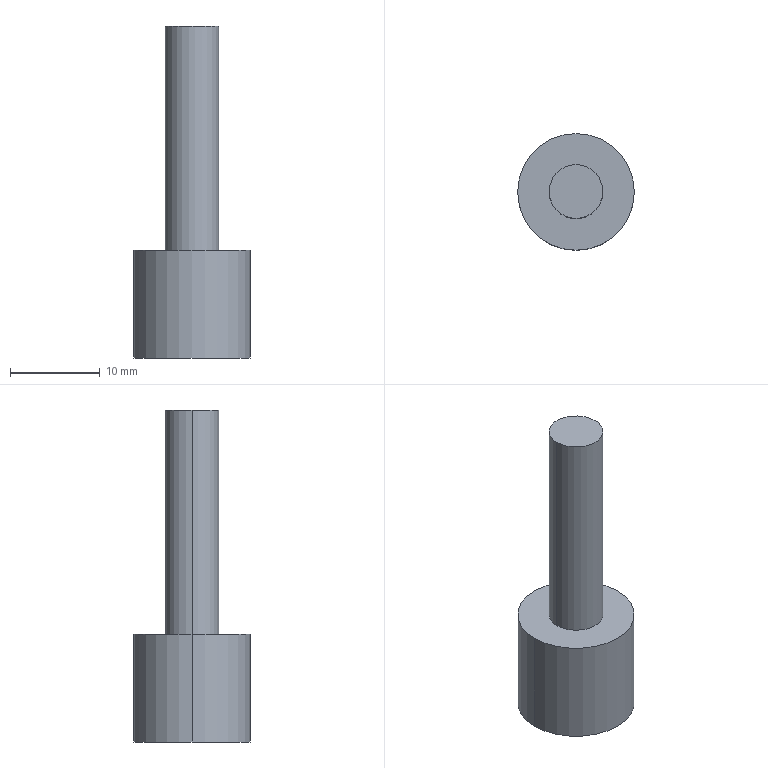Part | SolidWorks | features ICE 2, Extrusion 1 | 1 solid | 10 faces | box 13 x 13 x 37 mm | volume 2260 mm3 | cylinder 6 | plane 4 | commonest cylinder face diameters 6 x2 10 x2 13 x2
STEP:
#1=CARTESIAN_POINT('',(5.,0.,0.5));
#2=VERTEX_POINT('',#1);
#3=CARTESIAN_POINT('',(-5.,0.,0.5));
#4=VERTEX_POINT('',#3);
#5=CARTESIAN_POINT('',(0.,0.,0.5));
#6=DIRECTION('',(0.,0.,-1.));
#7=DIRECTION('',(-1.,0.,0.));
#8=AXIS2_PLACEMENT_3D('',#5,#6,#7);
#9=CIRCLE('',#8,5.);
#10=EDGE_CURVE('',#2,#4,#9,.T.);
#11=ORIENTED_EDGE('',*,*,#10,.F.);
#12=CARTESIAN_POINT('',(5.,0.,0.));
#13=VERTEX_POINT('',#12);
#14=CARTESIAN_POINT('',(5.,0.,0.5));
#15=DIRECTION('',(0.,0.,-1.));
#16=VECTOR('',#15,1000.);
#17=LINE('',#14,#16);
#18=EDGE_CURVE('',#2,#13,#17,.T.);
#19=ORIENTED_EDGE('',*,*,#18,.T.);
#20=CARTESIAN_POINT('',(-5.,0.,0.));
#21=VERTEX_POINT('',#20);
#22=CARTESIAN_POINT('',(0.,0.,0.));
#23=DIRECTION('',(0.,0.,-1.));
#24=DIRECTION('',(-1.,0.,0.));
#25=AXIS2_PLACEMENT_3D('',#22,#23,#24);
#26=CIRCLE('',#25,5.);
#27=EDGE_CURVE('',#13,#21,#26,.T.);
#28=ORIENTED_EDGE('',*,*,#27,.T.);
#29=CARTESIAN_POINT('',(-5.,0.,0.5));
#30=DIRECTION('',(0.,0.,-1.));
#31=VECTOR('',#30,1000.);
#32=LINE('',#29,#31);
#33=EDGE_CURVE('',#4,#21,#32,.T.);
#34=ORIENTED_EDGE('',*,*,#33,.F.);
#35=EDGE_LOOP('',(#11,#19,#28,#34));
#36=FACE_OUTER_BOUND('',#35,.T.);
#37=CARTESIAN_POINT('',(0.,0.,0.5));
#38=DIRECTION('',(0.,0.,-1.));
#39=DIRECTION('',(-1.,0.,0.));
#40=AXIS2_PLACEMENT_3D('',#37,#38,#39);
#41=CYLINDRICAL_SURFACE('',#40,5.);
#42=ADVANCED_FACE('',(#36),#41,.F.);
#43=CARTESIAN_POINT('',(3.,0.,37.));
#44=VERTEX_POINT('',#43);
#45=CARTESIAN_POINT('',(-3.,0.,37.));
#46=VERTEX_POINT('',#45);
#47=CARTESIAN_POINT('',(0.,0.,37.));
#48=DIRECTION('',(0.,0.,1.));
#49=DIRECTION('',(1.,0.,0.));
#50=AXIS2_PLACEMENT_3D('',#47,#48,#49);
#51=CIRCLE('',#50,3.);
#52=EDGE_CURVE('',#44,#46,#51,.T.);
#53=ORIENTED_EDGE('',*,*,#52,.F.);
#54=CARTESIAN_POINT('',(3.,0.,12.));
#55=VERTEX_POINT('',#54);
#56=CARTESIAN_POINT('',(3.,0.,37.));
#57=DIRECTION('',(0.,0.,-1.));
#58=VECTOR('',#57,1000.);
#59=LINE('',#56,#58);
#60=EDGE_CURVE('',#44,#55,#59,.T.);
#61=ORIENTED_EDGE('',*,*,#60,.T.);
#62=CARTESIAN_POINT('',(-3.,0.,12.));
#63=VERTEX_POINT('',#62);
#64=CARTESIAN_POINT('',(0.,0.,12.));
#65=DIRECTION('',(0.,0.,1.));
#66=DIRECTION('',(1.,0.,0.));
#67=AXIS2_PLACEMENT_3D('',#64,#65,#66);
#68=CIRCLE('',#67,3.);
#69=EDGE_CURVE('',#55,#63,#68,.T.);
#70=ORIENTED_EDGE('',*,*,#69,.T.);
#71=CARTESIAN_POINT('',(-3.,0.,37.));
#72=DIRECTION('',(0.,0.,-1.));
#73=VECTOR('',#72,1000.);
#74=LINE('',#71,#73);
#75=EDGE_CURVE('',#46,#63,#74,.T.);
#76=ORIENTED_EDGE('',*,*,#75,.F.);
#77=EDGE_LOOP('',(#53,#61,#70,#76));
#78=FACE_OUTER_BOUND('',#77,.T.);
#79=CARTESIAN_POINT('',(0.,0.,37.));
#80=DIRECTION('',(0.,0.,-1.));
#81=DIRECTION('',(-1.,0.,0.));
#82=AXIS2_PLACEMENT_3D('',#79,#80,#81);
#83=CYLINDRICAL_SURFACE('',#82,3.);
#84=ADVANCED_FACE('',(#78),#83,.T.);
#85=CARTESIAN_POINT('',(6.5,0.,12.));
#86=VERTEX_POINT('',#85);
#87=CARTESIAN_POINT('',(-6.5,0.,12.));
#88=VERTEX_POINT('',#87);
#89=CARTESIAN_POINT('',(0.,0.,12.));
#90=DIRECTION('',(0.,0.,1.));
#91=DIRECTION('',(1.,0.,0.));
#92=AXIS2_PLACEMENT_3D('',#89,#90,#91);
#93=CIRCLE('',#92,6.5);
#94=EDGE_CURVE('',#86,#88,#93,.T.);
#95=ORIENTED_EDGE('',*,*,#94,.F.);
#96=CARTESIAN_POINT('',(6.5,0.,0.));
#97=VERTEX_POINT('',#96);
#98=CARTESIAN_POINT('',(6.5,0.,12.));
#99=DIRECTION('',(0.,0.,-1.));
#100=VECTOR('',#99,1000.);
#101=LINE('',#98,#100);
#102=EDGE_CURVE('',#86,#97,#101,.T.);
#103=ORIENTED_EDGE('',*,*,#102,.T.);
#104=CARTESIAN_POINT('',(-6.5,0.,0.));
#105=VERTEX_POINT('',#104);
#106=CARTESIAN_POINT('',(0.,0.,0.));
#107=DIRECTION('',(0.,0.,1.));
#108=DIRECTION('',(1.,0.,0.));
#109=AXIS2_PLACEMENT_3D('',#106,#107,#108);
#110=CIRCLE('',#109,6.5);
#111=EDGE_CURVE('',#97,#105,#110,.T.);
#112=ORIENTED_EDGE('',*,*,#111,.T.);
#113=CARTESIAN_POINT('',(-6.5,0.,12.));
#114=DIRECTION('',(0.,0.,-1.));
#115=VECTOR('',#114,1000.);
#116=LINE('',#113,#115);
#117=EDGE_CURVE('',#88,#105,#116,.T.);
#118=ORIENTED_EDGE('',*,*,#117,.F.);
#119=EDGE_LOOP('',(#95,#103,#112,#118));
#120=FACE_OUTER_BOUND('',#119,.T.);
#121=CARTESIAN_POINT('',(0.,0.,12.));
#122=DIRECTION('',(0.,0.,-1.));
#123=DIRECTION('',(-1.,0.,0.));
#124=AXIS2_PLACEMENT_3D('',#121,#122,#123);
#125=CYLINDRICAL_SURFACE('',#124,6.5);
#126=ADVANCED_FACE('',(#120),#125,.T.);
#127=ORIENTED_EDGE('',*,*,#102,.F.);
#128=CARTESIAN_POINT('',(0.,0.,12.));
#129=DIRECTION('',(0.,0.,1.));
#130=DIRECTION('',(1.,0.,0.));
#131=AXIS2_PLACEMENT_3D('',#128,#129,#130);
#132=CIRCLE('',#131,6.5);
#133=EDGE_CURVE('',#88,#86,#132,.T.);
#134=ORIENTED_EDGE('',*,*,#133,.F.);
#135=ORIENTED_EDGE('',*,*,#117,.T.);
#136=CARTESIAN_POINT('',(0.,0.,0.));
#137=DIRECTION('',(0.,0.,1.));
#138=DIRECTION('',(1.,0.,0.));
#139=AXIS2_PLACEMENT_3D('',#136,#137,#138);
#140=CIRCLE('',#139,6.5);
#141=EDGE_CURVE('',#105,#97,#140,.T.);
#142=ORIENTED_EDGE('',*,*,#141,.T.);
#143=EDGE_LOOP('',(#127,#134,#135,#142));
#144=FACE_OUTER_BOUND('',#143,.T.);
#145=CARTESIAN_POINT('',(0.,0.,12.));
#146=DIRECTION('',(0.,0.,-1.));
#147=DIRECTION('',(-1.,0.,0.));
#148=AXIS2_PLACEMENT_3D('',#145,#146,#147);
#149=CYLINDRICAL_SURFACE('',#148,6.5);
#150=ADVANCED_FACE('',(#144),#149,.T.);
#151=CARTESIAN_POINT('',(0.,0.,12.));
#152=DIRECTION('',(0.,0.,1.));
#153=DIRECTION('',(1.,0.,0.));
#154=AXIS2_PLACEMENT_3D('',#151,#152,#153);
#155=CIRCLE('',#154,3.);
#156=EDGE_CURVE('',#63,#55,#155,.T.);
#157=ORIENTED_EDGE('',*,*,#156,.F.);
#158=ORIENTED_EDGE('',*,*,#69,.F.);
#159=EDGE_LOOP('',(#157,#158));
#160=FACE_BOUND('',#159,.T.);
#161=ORIENTED_EDGE('',*,*,#133,.T.);
#162=ORIENTED_EDGE('',*,*,#94,.T.);
#163=EDGE_LOOP('',(#161,#162));
#164=FACE_OUTER_BOUND('',#163,.T.);
#165=CARTESIAN_POINT('',(0.,0.,12.));
#166=DIRECTION('',(0.,0.,1.));
#167=DIRECTION('',(1.,0.,0.));
#168=AXIS2_PLACEMENT_3D('',#165,#166,#167);
#169=PLANE('',#168);
#170=ADVANCED_FACE('',(#160,#164),#169,.T.);
#171=CARTESIAN_POINT('',(0.,0.,0.));
#172=DIRECTION('',(0.,0.,-1.));
#173=DIRECTION('',(-1.,0.,0.));
#174=AXIS2_PLACEMENT_3D('',#171,#172,#173);
#175=CIRCLE('',#174,5.);
#176=EDGE_CURVE('',#21,#13,#175,.T.);
#177=ORIENTED_EDGE('',*,*,#176,.F.);
#178=ORIENTED_EDGE('',*,*,#27,.F.);
#179=EDGE_LOOP('',(#177,#178));
#180=FACE_BOUND('',#179,.T.);
#181=ORIENTED_EDGE('',*,*,#141,.F.);
#182=ORIENTED_EDGE('',*,*,#111,.F.);
#183=EDGE_LOOP('',(#181,#182));
#184=FACE_OUTER_BOUND('',#183,.T.);
#185=CARTESIAN_POINT('',(0.,0.,0.));
#186=DIRECTION('',(0.,0.,1.));
#187=DIRECTION('',(1.,0.,0.));
#188=AXIS2_PLACEMENT_3D('',#185,#186,#187);
#189=PLANE('',#188);
#190=ADVANCED_FACE('',(#180,#184),#189,.F.);
#191=ORIENTED_EDGE('',*,*,#60,.F.);
#192=CARTESIAN_POINT('',(0.,0.,37.));
#193=DIRECTION('',(0.,0.,1.));
#194=DIRECTION('',(1.,0.,0.));
#195=AXIS2_PLACEMENT_3D('',#192,#193,#194);
#196=CIRCLE('',#195,3.);
#197=EDGE_CURVE('',#46,#44,#196,.T.);
#198=ORIENTED_EDGE('',*,*,#197,.F.);
#199=ORIENTED_EDGE('',*,*,#75,.T.);
#200=ORIENTED_EDGE('',*,*,#156,.T.);
#201=EDGE_LOOP('',(#191,#198,#199,#200));
#202=FACE_OUTER_BOUND('',#201,.T.);
#203=CARTESIAN_POINT('',(0.,0.,37.));
#204=DIRECTION('',(0.,0.,-1.));
#205=DIRECTION('',(-1.,0.,0.));
#206=AXIS2_PLACEMENT_3D('',#203,#204,#205);
#207=CYLINDRICAL_SURFACE('',#206,3.);
#208=ADVANCED_FACE('',(#202),#207,.T.);
#209=ORIENTED_EDGE('',*,*,#197,.T.);
#210=ORIENTED_EDGE('',*,*,#52,.T.);
#211=EDGE_LOOP('',(#209,#210));
#212=FACE_OUTER_BOUND('',#211,.T.);
#213=CARTESIAN_POINT('',(0.,0.,37.));
#214=DIRECTION('',(0.,0.,1.));
#215=DIRECTION('',(1.,0.,0.));
#216=AXIS2_PLACEMENT_3D('',#213,#214,#215);
#217=PLANE('',#216);
#218=ADVANCED_FACE('',(#212),#217,.T.);
#219=ORIENTED_EDGE('',*,*,#18,.F.);
#220=CARTESIAN_POINT('',(0.,0.,0.5));
#221=DIRECTION('',(0.,0.,-1.));
#222=DIRECTION('',(-1.,0.,0.));
#223=AXIS2_PLACEMENT_3D('',#220,#221,#222);
#224=CIRCLE('',#223,5.);
#225=EDGE_CURVE('',#4,#2,#224,.T.);
#226=ORIENTED_EDGE('',*,*,#225,.F.);
#227=ORIENTED_EDGE('',*,*,#33,.T.);
#228=ORIENTED_EDGE('',*,*,#176,.T.);
#229=EDGE_LOOP('',(#219,#226,#227,#228));
#230=FACE_OUTER_BOUND('',#229,.T.);
#231=CARTESIAN_POINT('',(0.,0.,0.5));
#232=DIRECTION('',(0.,0.,-1.));
#233=DIRECTION('',(-1.,0.,0.));
#234=AXIS2_PLACEMENT_3D('',#231,#232,#233);
#235=CYLINDRICAL_SURFACE('',#234,5.);
#236=ADVANCED_FACE('',(#230),#235,.F.);
#237=ORIENTED_EDGE('',*,*,#225,.T.);
#238=ORIENTED_EDGE('',*,*,#10,.T.);
#239=EDGE_LOOP('',(#237,#238));
#240=FACE_OUTER_BOUND('',#239,.T.);
#241=CARTESIAN_POINT('',(0.,0.,0.5));
#242=DIRECTION('',(0.,0.,-1.));
#243=DIRECTION('',(-1.,0.,0.));
#244=AXIS2_PLACEMENT_3D('',#241,#242,#243);
#245=PLANE('',#244);
#246=ADVANCED_FACE('',(#240),#245,.T.);
#247=CLOSED_SHELL('',(#42,#84,#126,#150,#170,#190,#208,#218,#236,#246));
#248=MANIFOLD_SOLID_BREP('',#247);
#249=CARTESIAN_POINT('',(0.,0.,0.));
#250=DIRECTION('',(0.,0.,1.));
#251=DIRECTION('',(1.,0.,0.));
#252=AXIS2_PLACEMENT_3D('',#249,#250,#251);
#253=(LENGTH_UNIT()NAMED_UNIT(*)SI_UNIT(.MILLI.,.METRE.));
#254=UNCERTAINTY_MEASURE_WITH_UNIT(LENGTH_MEASURE(0.00001),#253,'','');
#255=(NAMED_UNIT(*)PLANE_ANGLE_UNIT()SI_UNIT($,.RADIAN.));
#256=(NAMED_UNIT(*)SI_UNIT($,.STERADIAN.)SOLID_ANGLE_UNIT());
#257=(GEOMETRIC_REPRESENTATION_CONTEXT(3)GLOBAL_UNCERTAINTY_ASSIGNED_CONTEXT((#254))GLOBAL_UNIT_ASSIGNED_CONTEXT((#253,#255,#256))REPRESENTATION_CONTEXT('',''));
#258=ADVANCED_BREP_SHAPE_REPRESENTATION('',(#248,#252),#257);